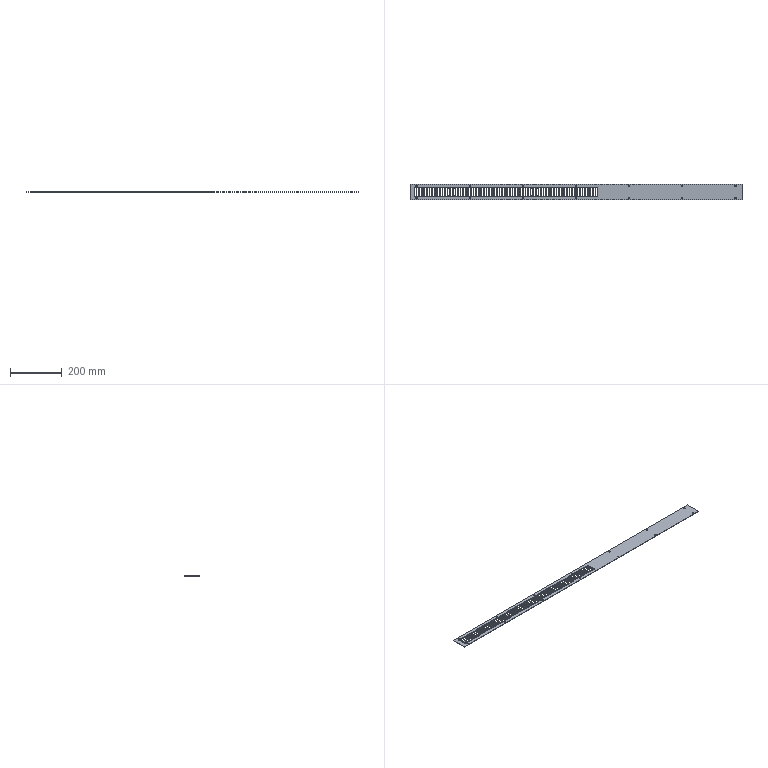Part | STEP file | 1 solid | 318 faces | box 1280 x 60 x 1.5 mm | volume 89815 mm3 | cylinder 170 | plane 148 | commonest cylinder face diameters 7 x142 5 x28